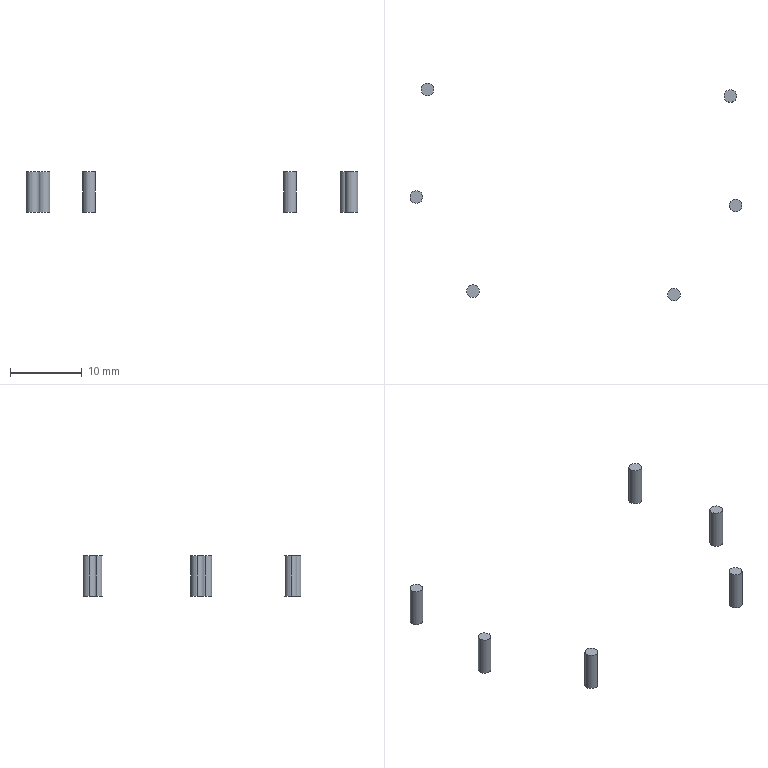Part | STEP file | TQ-DD-1105-THCoil1010_デフォルト | 6 solids | 24 faces | box 46.175 x 30.321 x 5.639 mm | volume 82.319 mm3 | cylinder 12 | plane 12 | commonest cylinder face diameters 1.76 x12
STEP:
#1=CARTESIAN_POINT('',(-23.276,-5.048,13.121));
#2=VERTEX_POINT('',#1);
#3=CARTESIAN_POINT('',(-21.516,-5.048,13.121));
#4=VERTEX_POINT('',#3);
#5=CARTESIAN_POINT('',(-22.396,-5.048,13.121));
#6=DIRECTION('',(0.,0.,-1.));
#7=DIRECTION('',(-0.8591,-0.5117,0.));
#8=AXIS2_PLACEMENT_3D('',#5,#6,#7);
#9=CIRCLE('',#8,0.88);
#10=EDGE_CURVE('',#2,#4,#9,.T.);
#11=ORIENTED_EDGE('',*,*,#10,.F.);
#12=CARTESIAN_POINT('',(-23.276,-5.048,18.76));
#13=VERTEX_POINT('',#12);
#14=CARTESIAN_POINT('',(-23.276,-5.048,8.76));
#15=DIRECTION('',(0.,0.,1.));
#16=VECTOR('',#15,1000.);
#17=LINE('',#14,#16);
#18=EDGE_CURVE('',#2,#13,#17,.T.);
#19=ORIENTED_EDGE('',*,*,#18,.T.);
#20=CARTESIAN_POINT('',(-21.516,-5.048,18.76));
#21=VERTEX_POINT('',#20);
#22=CARTESIAN_POINT('',(-22.396,-5.048,18.76));
#23=DIRECTION('',(0.,0.,-1.));
#24=DIRECTION('',(1.,0.,0.));
#25=AXIS2_PLACEMENT_3D('',#22,#23,#24);
#26=CIRCLE('',#25,0.88);
#27=EDGE_CURVE('',#13,#21,#26,.T.);
#28=ORIENTED_EDGE('',*,*,#27,.T.);
#29=CARTESIAN_POINT('',(-21.516,-5.048,8.76));
#30=DIRECTION('',(0.,0.,1.));
#31=VECTOR('',#30,1000.);
#32=LINE('',#29,#31);
#33=EDGE_CURVE('',#4,#21,#32,.T.);
#34=ORIENTED_EDGE('',*,*,#33,.F.);
#35=EDGE_LOOP('',(#11,#19,#28,#34));
#36=FACE_OUTER_BOUND('',#35,.T.);
#37=CARTESIAN_POINT('',(-22.396,-5.048,8.76));
#38=DIRECTION('',(0.,0.,1.));
#39=DIRECTION('',(1.,0.,0.));
#40=AXIS2_PLACEMENT_3D('',#37,#38,#39);
#41=CYLINDRICAL_SURFACE('',#40,0.88);
#42=ADVANCED_FACE('',(#36),#41,.T.);
#43=ORIENTED_EDGE('',*,*,#18,.F.);
#44=CARTESIAN_POINT('',(-22.396,-5.048,13.121));
#45=DIRECTION('',(0.,0.,-1.));
#46=DIRECTION('',(-0.8591,-0.5117,0.));
#47=AXIS2_PLACEMENT_3D('',#44,#45,#46);
#48=CIRCLE('',#47,0.88);
#49=EDGE_CURVE('',#4,#2,#48,.T.);
#50=ORIENTED_EDGE('',*,*,#49,.F.);
#51=ORIENTED_EDGE('',*,*,#33,.T.);
#52=CARTESIAN_POINT('',(-22.396,-5.048,18.76));
#53=DIRECTION('',(0.,0.,-1.));
#54=DIRECTION('',(1.,0.,0.));
#55=AXIS2_PLACEMENT_3D('',#52,#53,#54);
#56=CIRCLE('',#55,0.88);
#57=EDGE_CURVE('',#21,#13,#56,.T.);
#58=ORIENTED_EDGE('',*,*,#57,.T.);
#59=EDGE_LOOP('',(#43,#50,#51,#58));
#60=FACE_OUTER_BOUND('',#59,.T.);
#61=CARTESIAN_POINT('',(-22.396,-5.048,8.76));
#62=DIRECTION('',(0.,0.,1.));
#63=DIRECTION('',(1.,0.,0.));
#64=AXIS2_PLACEMENT_3D('',#61,#62,#63);
#65=CYLINDRICAL_SURFACE('',#64,0.88);
#66=ADVANCED_FACE('',(#60),#65,.T.);
#67=ORIENTED_EDGE('',*,*,#57,.F.);
#68=ORIENTED_EDGE('',*,*,#27,.F.);
#69=EDGE_LOOP('',(#67,#68));
#70=FACE_OUTER_BOUND('',#69,.T.);
#71=CARTESIAN_POINT('',(0.,0.,18.76));
#72=DIRECTION('',(0.,0.,1.));
#73=DIRECTION('',(1.,0.,0.));
#74=AXIS2_PLACEMENT_3D('',#71,#72,#73);
#75=PLANE('',#74);
#76=ADVANCED_FACE('',(#70),#75,.T.);
#77=ORIENTED_EDGE('',*,*,#49,.T.);
#78=ORIENTED_EDGE('',*,*,#10,.T.);
#79=EDGE_LOOP('',(#77,#78));
#80=FACE_OUTER_BOUND('',#79,.T.);
#81=CARTESIAN_POINT('',(48.882,-17.585,13.121));
#82=DIRECTION('',(0.,0.,1.));
#83=DIRECTION('',(-0.8591,-0.5117,0.));
#84=AXIS2_PLACEMENT_3D('',#81,#82,#83);
#85=PLANE('',#84);
#86=ADVANCED_FACE('',(#80),#85,.F.);
#87=CLOSED_SHELL('',(#42,#66,#76,#86));
#88=MANIFOLD_SOLID_BREP('',#87);
#89=CARTESIAN_POINT('',(-15.383,-18.145,13.121));
#90=VERTEX_POINT('',#89);
#91=CARTESIAN_POINT('',(-13.623,-18.145,13.121));
#92=VERTEX_POINT('',#91);
#93=CARTESIAN_POINT('',(-14.503,-18.145,13.121));
#94=DIRECTION('',(0.,0.,-1.));
#95=DIRECTION('',(-0.8591,-0.5117,0.));
#96=AXIS2_PLACEMENT_3D('',#93,#94,#95);
#97=CIRCLE('',#96,0.88);
#98=EDGE_CURVE('',#90,#92,#97,.T.);
#99=ORIENTED_EDGE('',*,*,#98,.F.);
#100=CARTESIAN_POINT('',(-15.383,-18.145,18.76));
#101=VERTEX_POINT('',#100);
#102=CARTESIAN_POINT('',(-15.383,-18.145,8.76));
#103=DIRECTION('',(0.,0.,1.));
#104=VECTOR('',#103,1000.);
#105=LINE('',#102,#104);
#106=EDGE_CURVE('',#90,#101,#105,.T.);
#107=ORIENTED_EDGE('',*,*,#106,.T.);
#108=CARTESIAN_POINT('',(-13.623,-18.145,18.76));
#109=VERTEX_POINT('',#108);
#110=CARTESIAN_POINT('',(-14.503,-18.145,18.76));
#111=DIRECTION('',(0.,0.,-1.));
#112=DIRECTION('',(1.,0.,0.));
#113=AXIS2_PLACEMENT_3D('',#110,#111,#112);
#114=CIRCLE('',#113,0.88);
#115=EDGE_CURVE('',#101,#109,#114,.T.);
#116=ORIENTED_EDGE('',*,*,#115,.T.);
#117=CARTESIAN_POINT('',(-13.623,-18.145,8.76));
#118=DIRECTION('',(0.,0.,1.));
#119=VECTOR('',#118,1000.);
#120=LINE('',#117,#119);
#121=EDGE_CURVE('',#92,#109,#120,.T.);
#122=ORIENTED_EDGE('',*,*,#121,.F.);
#123=EDGE_LOOP('',(#99,#107,#116,#122));
#124=FACE_OUTER_BOUND('',#123,.T.);
#125=CARTESIAN_POINT('',(-14.503,-18.145,8.76));
#126=DIRECTION('',(0.,0.,1.));
#127=DIRECTION('',(1.,0.,0.));
#128=AXIS2_PLACEMENT_3D('',#125,#126,#127);
#129=CYLINDRICAL_SURFACE('',#128,0.88);
#130=ADVANCED_FACE('',(#124),#129,.T.);
#131=ORIENTED_EDGE('',*,*,#106,.F.);
#132=CARTESIAN_POINT('',(-14.503,-18.145,13.121));
#133=DIRECTION('',(0.,0.,-1.));
#134=DIRECTION('',(-0.8591,-0.5117,0.));
#135=AXIS2_PLACEMENT_3D('',#132,#133,#134);
#136=CIRCLE('',#135,0.88);
#137=EDGE_CURVE('',#92,#90,#136,.T.);
#138=ORIENTED_EDGE('',*,*,#137,.F.);
#139=ORIENTED_EDGE('',*,*,#121,.T.);
#140=CARTESIAN_POINT('',(-14.503,-18.145,18.76));
#141=DIRECTION('',(0.,0.,-1.));
#142=DIRECTION('',(1.,0.,0.));
#143=AXIS2_PLACEMENT_3D('',#140,#141,#142);
#144=CIRCLE('',#143,0.88);
#145=EDGE_CURVE('',#109,#101,#144,.T.);
#146=ORIENTED_EDGE('',*,*,#145,.T.);
#147=EDGE_LOOP('',(#131,#138,#139,#146));
#148=FACE_OUTER_BOUND('',#147,.T.);
#149=CARTESIAN_POINT('',(-14.503,-18.145,8.76));
#150=DIRECTION('',(0.,0.,1.));
#151=DIRECTION('',(1.,0.,0.));
#152=AXIS2_PLACEMENT_3D('',#149,#150,#151);
#153=CYLINDRICAL_SURFACE('',#152,0.88);
#154=ADVANCED_FACE('',(#148),#153,.T.);
#155=ORIENTED_EDGE('',*,*,#145,.F.);
#156=ORIENTED_EDGE('',*,*,#115,.F.);
#157=EDGE_LOOP('',(#155,#156));
#158=FACE_OUTER_BOUND('',#157,.T.);
#159=CARTESIAN_POINT('',(0.,0.,18.76));
#160=DIRECTION('',(0.,0.,1.));
#161=DIRECTION('',(1.,0.,0.));
#162=AXIS2_PLACEMENT_3D('',#159,#160,#161);
#163=PLANE('',#162);
#164=ADVANCED_FACE('',(#158),#163,.T.);
#165=ORIENTED_EDGE('',*,*,#137,.T.);
#166=ORIENTED_EDGE('',*,*,#98,.T.);
#167=EDGE_LOOP('',(#165,#166));
#168=FACE_OUTER_BOUND('',#167,.T.);
#169=CARTESIAN_POINT('',(48.882,-17.585,13.121));
#170=DIRECTION('',(0.,0.,1.));
#171=DIRECTION('',(-0.8591,-0.5117,0.));
#172=AXIS2_PLACEMENT_3D('',#169,#170,#171);
#173=PLANE('',#172);
#174=ADVANCED_FACE('',(#168),#173,.F.);
#175=CLOSED_SHELL('',(#130,#154,#164,#174));
#176=MANIFOLD_SOLID_BREP('',#175);
#177=CARTESIAN_POINT('',(20.411,8.991,13.121));
#178=VERTEX_POINT('',#177);
#179=CARTESIAN_POINT('',(22.171,8.991,13.121));
#180=VERTEX_POINT('',#179);
#181=CARTESIAN_POINT('',(21.291,8.991,13.121));
#182=DIRECTION('',(0.,0.,-1.));
#183=DIRECTION('',(-0.8591,-0.5117,0.));
#184=AXIS2_PLACEMENT_3D('',#181,#182,#183);
#185=CIRCLE('',#184,0.88);
#186=EDGE_CURVE('',#178,#180,#185,.T.);
#187=ORIENTED_EDGE('',*,*,#186,.F.);
#188=CARTESIAN_POINT('',(20.411,8.991,18.76));
#189=VERTEX_POINT('',#188);
#190=CARTESIAN_POINT('',(20.411,8.991,8.76));
#191=DIRECTION('',(0.,0.,1.));
#192=VECTOR('',#191,1000.);
#193=LINE('',#190,#192);
#194=EDGE_CURVE('',#178,#189,#193,.T.);
#195=ORIENTED_EDGE('',*,*,#194,.T.);
#196=CARTESIAN_POINT('',(22.171,8.991,18.76));
#197=VERTEX_POINT('',#196);
#198=CARTESIAN_POINT('',(21.291,8.991,18.76));
#199=DIRECTION('',(0.,0.,-1.));
#200=DIRECTION('',(1.,0.,0.));
#201=AXIS2_PLACEMENT_3D('',#198,#199,#200);
#202=CIRCLE('',#201,0.88);
#203=EDGE_CURVE('',#189,#197,#202,.T.);
#204=ORIENTED_EDGE('',*,*,#203,.T.);
#205=CARTESIAN_POINT('',(22.171,8.991,8.76));
#206=DIRECTION('',(0.,0.,1.));
#207=VECTOR('',#206,1000.);
#208=LINE('',#205,#207);
#209=EDGE_CURVE('',#180,#197,#208,.T.);
#210=ORIENTED_EDGE('',*,*,#209,.F.);
#211=EDGE_LOOP('',(#187,#195,#204,#210));
#212=FACE_OUTER_BOUND('',#211,.T.);
#213=CARTESIAN_POINT('',(21.291,8.991,8.76));
#214=DIRECTION('',(0.,0.,1.));
#215=DIRECTION('',(1.,0.,0.));
#216=AXIS2_PLACEMENT_3D('',#213,#214,#215);
#217=CYLINDRICAL_SURFACE('',#216,0.88);
#218=ADVANCED_FACE('',(#212),#217,.T.);
#219=ORIENTED_EDGE('',*,*,#194,.F.);
#220=CARTESIAN_POINT('',(21.291,8.991,13.121));
#221=DIRECTION('',(0.,0.,-1.));
#222=DIRECTION('',(-0.8591,-0.5117,0.));
#223=AXIS2_PLACEMENT_3D('',#220,#221,#222);
#224=CIRCLE('',#223,0.88);
#225=EDGE_CURVE('',#180,#178,#224,.T.);
#226=ORIENTED_EDGE('',*,*,#225,.F.);
#227=ORIENTED_EDGE('',*,*,#209,.T.);
#228=CARTESIAN_POINT('',(21.291,8.991,18.76));
#229=DIRECTION('',(0.,0.,-1.));
#230=DIRECTION('',(1.,0.,0.));
#231=AXIS2_PLACEMENT_3D('',#228,#229,#230);
#232=CIRCLE('',#231,0.88);
#233=EDGE_CURVE('',#197,#189,#232,.T.);
#234=ORIENTED_EDGE('',*,*,#233,.T.);
#235=EDGE_LOOP('',(#219,#226,#227,#234));
#236=FACE_OUTER_BOUND('',#235,.T.);
#237=CARTESIAN_POINT('',(21.291,8.991,8.76));
#238=DIRECTION('',(0.,0.,1.));
#239=DIRECTION('',(1.,0.,0.));
#240=AXIS2_PLACEMENT_3D('',#237,#238,#239);
#241=CYLINDRICAL_SURFACE('',#240,0.88);
#242=ADVANCED_FACE('',(#236),#241,.T.);
#243=ORIENTED_EDGE('',*,*,#233,.F.);
#244=ORIENTED_EDGE('',*,*,#203,.F.);
#245=EDGE_LOOP('',(#243,#244));
#246=FACE_OUTER_BOUND('',#245,.T.);
#247=CARTESIAN_POINT('',(0.,0.,18.76));
#248=DIRECTION('',(0.,0.,1.));
#249=DIRECTION('',(1.,0.,0.));
#250=AXIS2_PLACEMENT_3D('',#247,#248,#249);
#251=PLANE('',#250);
#252=ADVANCED_FACE('',(#246),#251,.T.);
#253=ORIENTED_EDGE('',*,*,#225,.T.);
#254=ORIENTED_EDGE('',*,*,#186,.T.);
#255=EDGE_LOOP('',(#253,#254));
#256=FACE_OUTER_BOUND('',#255,.T.);
#257=CARTESIAN_POINT('',(48.882,-17.585,13.121));
#258=DIRECTION('',(0.,0.,1.));
#259=DIRECTION('',(-0.8591,-0.5117,0.));
#260=AXIS2_PLACEMENT_3D('',#257,#258,#259);
#261=PLANE('',#260);
#262=ADVANCED_FACE('',(#256),#261,.F.);
#263=CLOSED_SHELL('',(#218,#242,#252,#262));
#264=MANIFOLD_SOLID_BREP('',#263);
#265=CARTESIAN_POINT('',(-21.725,9.932,13.121));
#266=VERTEX_POINT('',#265);
#267=CARTESIAN_POINT('',(-19.965,9.932,13.121));
#268=VERTEX_POINT('',#267);
#269=CARTESIAN_POINT('',(-20.845,9.932,13.121));
#270=DIRECTION('',(0.,0.,-1.));
#271=DIRECTION('',(-0.8591,-0.5117,0.));
#272=AXIS2_PLACEMENT_3D('',#269,#270,#271);
#273=CIRCLE('',#272,0.88);
#274=EDGE_CURVE('',#266,#268,#273,.T.);
#275=ORIENTED_EDGE('',*,*,#274,.F.);
#276=CARTESIAN_POINT('',(-21.725,9.932,18.76));
#277=VERTEX_POINT('',#276);
#278=CARTESIAN_POINT('',(-21.725,9.932,8.76));
#279=DIRECTION('',(0.,0.,1.));
#280=VECTOR('',#279,1000.);
#281=LINE('',#278,#280);
#282=EDGE_CURVE('',#266,#277,#281,.T.);
#283=ORIENTED_EDGE('',*,*,#282,.T.);
#284=CARTESIAN_POINT('',(-19.965,9.932,18.76));
#285=VERTEX_POINT('',#284);
#286=CARTESIAN_POINT('',(-20.845,9.932,18.76));
#287=DIRECTION('',(0.,0.,-1.));
#288=DIRECTION('',(1.,0.,0.));
#289=AXIS2_PLACEMENT_3D('',#286,#287,#288);
#290=CIRCLE('',#289,0.88);
#291=EDGE_CURVE('',#277,#285,#290,.T.);
#292=ORIENTED_EDGE('',*,*,#291,.T.);
#293=CARTESIAN_POINT('',(-19.965,9.932,8.76));
#294=DIRECTION('',(0.,0.,1.));
#295=VECTOR('',#294,1000.);
#296=LINE('',#293,#295);
#297=EDGE_CURVE('',#268,#285,#296,.T.);
#298=ORIENTED_EDGE('',*,*,#297,.F.);
#299=EDGE_LOOP('',(#275,#283,#292,#298));
#300=FACE_OUTER_BOUND('',#299,.T.);
#301=CARTESIAN_POINT('',(-20.845,9.932,8.76));
#302=DIRECTION('',(0.,0.,1.));
#303=DIRECTION('',(1.,0.,0.));
#304=AXIS2_PLACEMENT_3D('',#301,#302,#303);
#305=CYLINDRICAL_SURFACE('',#304,0.88);
#306=ADVANCED_FACE('',(#300),#305,.T.);
#307=ORIENTED_EDGE('',*,*,#282,.F.);
#308=CARTESIAN_POINT('',(-20.845,9.932,13.121));
#309=DIRECTION('',(0.,0.,-1.));
#310=DIRECTION('',(-0.8591,-0.5117,0.));
#311=AXIS2_PLACEMENT_3D('',#308,#309,#310);
#312=CIRCLE('',#311,0.88);
#313=EDGE_CURVE('',#268,#266,#312,.T.);
#314=ORIENTED_EDGE('',*,*,#313,.F.);
#315=ORIENTED_EDGE('',*,*,#297,.T.);
#316=CARTESIAN_POINT('',(-20.845,9.932,18.76));
#317=DIRECTION('',(0.,0.,-1.));
#318=DIRECTION('',(1.,0.,0.));
#319=AXIS2_PLACEMENT_3D('',#316,#317,#318);
#320=CIRCLE('',#319,0.88);
#321=EDGE_CURVE('',#285,#277,#320,.T.);
#322=ORIENTED_EDGE('',*,*,#321,.T.);
#323=EDGE_LOOP('',(#307,#314,#315,#322));
#324=FACE_OUTER_BOUND('',#323,.T.);
#325=CARTESIAN_POINT('',(-20.845,9.932,8.76));
#326=DIRECTION('',(0.,0.,1.));
#327=DIRECTION('',(1.,0.,0.));
#328=AXIS2_PLACEMENT_3D('',#325,#326,#327);
#329=CYLINDRICAL_SURFACE('',#328,0.88);
#330=ADVANCED_FACE('',(#324),#329,.T.);
#331=ORIENTED_EDGE('',*,*,#321,.F.);
#332=ORIENTED_EDGE('',*,*,#291,.F.);
#333=EDGE_LOOP('',(#331,#332));
#334=FACE_OUTER_BOUND('',#333,.T.);
#335=CARTESIAN_POINT('',(0.,0.,18.76));
#336=DIRECTION('',(0.,0.,1.));
#337=DIRECTION('',(1.,0.,0.));
#338=AXIS2_PLACEMENT_3D('',#335,#336,#337);
#339=PLANE('',#338);
#340=ADVANCED_FACE('',(#334),#339,.T.);
#341=ORIENTED_EDGE('',*,*,#313,.T.);
#342=ORIENTED_EDGE('',*,*,#274,.T.);
#343=EDGE_LOOP('',(#341,#342));
#344=FACE_OUTER_BOUND('',#343,.T.);
#345=CARTESIAN_POINT('',(48.882,-17.585,13.121));
#346=DIRECTION('',(0.,0.,1.));
#347=DIRECTION('',(-0.8591,-0.5117,0.));
#348=AXIS2_PLACEMENT_3D('',#345,#346,#347);
#349=PLANE('',#348);
#350=ADVANCED_FACE('',(#344),#349,.F.);
#351=CLOSED_SHELL('',(#306,#330,#340,#350));
#352=MANIFOLD_SOLID_BREP('',#351);
#353=CARTESIAN_POINT('',(12.554,-18.629,13.121));
#354=VERTEX_POINT('',#353);
#355=CARTESIAN_POINT('',(14.314,-18.629,13.121));
#356=VERTEX_POINT('',#355);
#357=CARTESIAN_POINT('',(13.434,-18.629,13.121));
#358=DIRECTION('',(0.,0.,-1.));
#359=DIRECTION('',(-0.8591,-0.5117,0.));
#360=AXIS2_PLACEMENT_3D('',#357,#358,#359);
#361=CIRCLE('',#360,0.88);
#362=EDGE_CURVE('',#354,#356,#361,.T.);
#363=ORIENTED_EDGE('',*,*,#362,.F.);
#364=CARTESIAN_POINT('',(12.554,-18.629,18.76));
#365=VERTEX_POINT('',#364);
#366=CARTESIAN_POINT('',(12.554,-18.629,8.76));
#367=DIRECTION('',(0.,0.,1.));
#368=VECTOR('',#367,1000.);
#369=LINE('',#366,#368);
#370=EDGE_CURVE('',#354,#365,#369,.T.);
#371=ORIENTED_EDGE('',*,*,#370,.T.);
#372=CARTESIAN_POINT('',(14.314,-18.629,18.76));
#373=VERTEX_POINT('',#372);
#374=CARTESIAN_POINT('',(13.434,-18.629,18.76));
#375=DIRECTION('',(0.,0.,-1.));
#376=DIRECTION('',(1.,0.,0.));
#377=AXIS2_PLACEMENT_3D('',#374,#375,#376);
#378=CIRCLE('',#377,0.88);
#379=EDGE_CURVE('',#365,#373,#378,.T.);
#380=ORIENTED_EDGE('',*,*,#379,.T.);
#381=CARTESIAN_POINT('',(14.314,-18.629,8.76));
#382=DIRECTION('',(0.,0.,1.));
#383=VECTOR('',#382,1000.);
#384=LINE('',#381,#383);
#385=EDGE_CURVE('',#356,#373,#384,.T.);
#386=ORIENTED_EDGE('',*,*,#385,.F.);
#387=EDGE_LOOP('',(#363,#371,#380,#386));
#388=FACE_OUTER_BOUND('',#387,.T.);
#389=CARTESIAN_POINT('',(13.434,-18.629,8.76));
#390=DIRECTION('',(0.,0.,1.));
#391=DIRECTION('',(1.,0.,0.));
#392=AXIS2_PLACEMENT_3D('',#389,#390,#391);
#393=CYLINDRICAL_SURFACE('',#392,0.88);
#394=ADVANCED_FACE('',(#388),#393,.T.);
#395=ORIENTED_EDGE('',*,*,#370,.F.);
#396=CARTESIAN_POINT('',(13.434,-18.629,13.121));
#397=DIRECTION('',(0.,0.,-1.));
#398=DIRECTION('',(-0.8591,-0.5117,0.));
#399=AXIS2_PLACEMENT_3D('',#396,#397,#398);
#400=CIRCLE('',#399,0.88);
#401=EDGE_CURVE('',#356,#354,#400,.T.);
#402=ORIENTED_EDGE('',*,*,#401,.F.);
#403=ORIENTED_EDGE('',*,*,#385,.T.);
#404=CARTESIAN_POINT('',(13.434,-18.629,18.76));
#405=DIRECTION('',(0.,0.,-1.));
#406=DIRECTION('',(1.,0.,0.));
#407=AXIS2_PLACEMENT_3D('',#404,#405,#406);
#408=CIRCLE('',#407,0.88);
#409=EDGE_CURVE('',#373,#365,#408,.T.);
#410=ORIENTED_EDGE('',*,*,#409,.T.);
#411=EDGE_LOOP('',(#395,#402,#403,#410));
#412=FACE_OUTER_BOUND('',#411,.T.);
#413=CARTESIAN_POINT('',(13.434,-18.629,8.76));
#414=DIRECTION('',(0.,0.,1.));
#415=DIRECTION('',(1.,0.,0.));
#416=AXIS2_PLACEMENT_3D('',#413,#414,#415);
#417=CYLINDRICAL_SURFACE('',#416,0.88);
#418=ADVANCED_FACE('',(#412),#417,.T.);
#419=ORIENTED_EDGE('',*,*,#409,.F.);
#420=ORIENTED_EDGE('',*,*,#379,.F.);
#421=EDGE_LOOP('',(#419,#420));
#422=FACE_OUTER_BOUND('',#421,.T.);
#423=CARTESIAN_POINT('',(0.,0.,18.76));
#424=DIRECTION('',(0.,0.,1.));
#425=DIRECTION('',(1.,0.,0.));
#426=AXIS2_PLACEMENT_3D('',#423,#424,#425);
#427=PLANE('',#426);
#428=ADVANCED_FACE('',(#422),#427,.T.);
#429=ORIENTED_EDGE('',*,*,#401,.T.);
#430=ORIENTED_EDGE('',*,*,#362,.T.);
#431=EDGE_LOOP('',(#429,#430));
#432=FACE_OUTER_BOUND('',#431,.T.);
#433=CARTESIAN_POINT('',(48.882,-17.585,13.121));
#434=DIRECTION('',(0.,0.,1.));
#435=DIRECTION('',(-0.8591,-0.5117,0.));
#436=AXIS2_PLACEMENT_3D('',#433,#434,#435);
#437=PLANE('',#436);
#438=ADVANCED_FACE('',(#432),#437,.F.);
#439=CLOSED_SHELL('',(#394,#418,#428,#438));
#440=MANIFOLD_SOLID_BREP('',#439);
#441=CARTESIAN_POINT('',(21.138,-6.225,13.121));
#442=VERTEX_POINT('',#441);
#443=CARTESIAN_POINT('',(22.898,-6.225,13.121));
#444=VERTEX_POINT('',#443);
#445=CARTESIAN_POINT('',(22.018,-6.225,13.121));
#446=DIRECTION('',(0.,0.,-1.));
#447=DIRECTION('',(-0.8591,-0.5117,0.));
#448=AXIS2_PLACEMENT_3D('',#445,#446,#447);
#449=CIRCLE('',#448,0.88);
#450=EDGE_CURVE('',#442,#444,#449,.T.);
#451=ORIENTED_EDGE('',*,*,#450,.F.);
#452=CARTESIAN_POINT('',(21.138,-6.225,18.76));
#453=VERTEX_POINT('',#452);
#454=CARTESIAN_POINT('',(21.138,-6.225,8.76));
#455=DIRECTION('',(0.,0.,1.));
#456=VECTOR('',#455,1000.);
#457=LINE('',#454,#456);
#458=EDGE_CURVE('',#442,#453,#457,.T.);
#459=ORIENTED_EDGE('',*,*,#458,.T.);
#460=CARTESIAN_POINT('',(22.898,-6.225,18.76));
#461=VERTEX_POINT('',#460);
#462=CARTESIAN_POINT('',(22.018,-6.225,18.76));
#463=DIRECTION('',(0.,0.,-1.));
#464=DIRECTION('',(1.,0.,0.));
#465=AXIS2_PLACEMENT_3D('',#462,#463,#464);
#466=CIRCLE('',#465,0.88);
#467=EDGE_CURVE('',#453,#461,#466,.T.);
#468=ORIENTED_EDGE('',*,*,#467,.T.);
#469=CARTESIAN_POINT('',(22.898,-6.225,8.76));
#470=DIRECTION('',(0.,0.,1.));
#471=VECTOR('',#470,1000.);
#472=LINE('',#469,#471);
#473=EDGE_CURVE('',#444,#461,#472,.T.);
#474=ORIENTED_EDGE('',*,*,#473,.F.);
#475=EDGE_LOOP('',(#451,#459,#468,#474));
#476=FACE_OUTER_BOUND('',#475,.T.);
#477=CARTESIAN_POINT('',(22.018,-6.225,8.76));
#478=DIRECTION('',(0.,0.,1.));
#479=DIRECTION('',(1.,0.,0.));
#480=AXIS2_PLACEMENT_3D('',#477,#478,#479);
#481=CYLINDRICAL_SURFACE('',#480,0.88);
#482=ADVANCED_FACE('',(#476),#481,.T.);
#483=ORIENTED_EDGE('',*,*,#458,.F.);
#484=CARTESIAN_POINT('',(22.018,-6.225,13.121));
#485=DIRECTION('',(0.,0.,-1.));
#486=DIRECTION('',(-0.8591,-0.5117,0.));
#487=AXIS2_PLACEMENT_3D('',#484,#485,#486);
#488=CIRCLE('',#487,0.88);
#489=EDGE_CURVE('',#444,#442,#488,.T.);
#490=ORIENTED_EDGE('',*,*,#489,.F.);
#491=ORIENTED_EDGE('',*,*,#473,.T.);
#492=CARTESIAN_POINT('',(22.018,-6.225,18.76));
#493=DIRECTION('',(0.,0.,-1.));
#494=DIRECTION('',(1.,0.,0.));
#495=AXIS2_PLACEMENT_3D('',#492,#493,#494);
#496=CIRCLE('',#495,0.88);
#497=EDGE_CURVE('',#461,#453,#496,.T.);
#498=ORIENTED_EDGE('',*,*,#497,.T.);
#499=EDGE_LOOP('',(#483,#490,#491,#498));
#500=FACE_OUTER_BOUND('',#499,.T.);
#501=CARTESIAN_POINT('',(22.018,-6.225,8.76));
#502=DIRECTION('',(0.,0.,1.));
#503=DIRECTION('',(1.,0.,0.));
#504=AXIS2_PLACEMENT_3D('',#501,#502,#503);
#505=CYLINDRICAL_SURFACE('',#504,0.88);
#506=ADVANCED_FACE('',(#500),#505,.T.);
#507=ORIENTED_EDGE('',*,*,#497,.F.);
#508=ORIENTED_EDGE('',*,*,#467,.F.);
#509=EDGE_LOOP('',(#507,#508));
#510=FACE_OUTER_BOUND('',#509,.T.);
#511=CARTESIAN_POINT('',(0.,0.,18.76));
#512=DIRECTION('',(0.,0.,1.));
#513=DIRECTION('',(1.,0.,0.));
#514=AXIS2_PLACEMENT_3D('',#511,#512,#513);
#515=PLANE('',#514);
#516=ADVANCED_FACE('',(#510),#515,.T.);
#517=ORIENTED_EDGE('',*,*,#489,.T.);
#518=ORIENTED_EDGE('',*,*,#450,.T.);
#519=EDGE_LOOP('',(#517,#518));
#520=FACE_OUTER_BOUND('',#519,.T.);
#521=CARTESIAN_POINT('',(48.882,-17.585,13.121));
#522=DIRECTION('',(0.,0.,1.));
#523=DIRECTION('',(-0.8591,-0.5117,0.));
#524=AXIS2_PLACEMENT_3D('',#521,#522,#523);
#525=PLANE('',#524);
#526=ADVANCED_FACE('',(#520),#525,.F.);
#527=CLOSED_SHELL('',(#482,#506,#516,#526));
#528=MANIFOLD_SOLID_BREP('',#527);
#529=CARTESIAN_POINT('',(0.,0.,0.));
#530=DIRECTION('',(0.,0.,1.));
#531=DIRECTION('',(1.,0.,0.));
#532=AXIS2_PLACEMENT_3D('',#529,#530,#531);
#533=(LENGTH_UNIT()NAMED_UNIT(*)SI_UNIT(.MILLI.,.METRE.));
#534=UNCERTAINTY_MEASURE_WITH_UNIT(LENGTH_MEASURE(0.00001),#533,'','');
#535=(NAMED_UNIT(*)PLANE_ANGLE_UNIT()SI_UNIT($,.RADIAN.));
#536=(NAMED_UNIT(*)SI_UNIT($,.STERADIAN.)SOLID_ANGLE_UNIT());
#537=(GEOMETRIC_REPRESENTATION_CONTEXT(3)GLOBAL_UNCERTAINTY_ASSIGNED_CONTEXT((#534))GLOBAL_UNIT_ASSIGNED_CONTEXT((#533,#535,#536))REPRESENTATION_CONTEXT('',''));
#538=ADVANCED_BREP_SHAPE_REPRESENTATION('',(#88,#176,#264,#352,#440,#528,#532),#537);